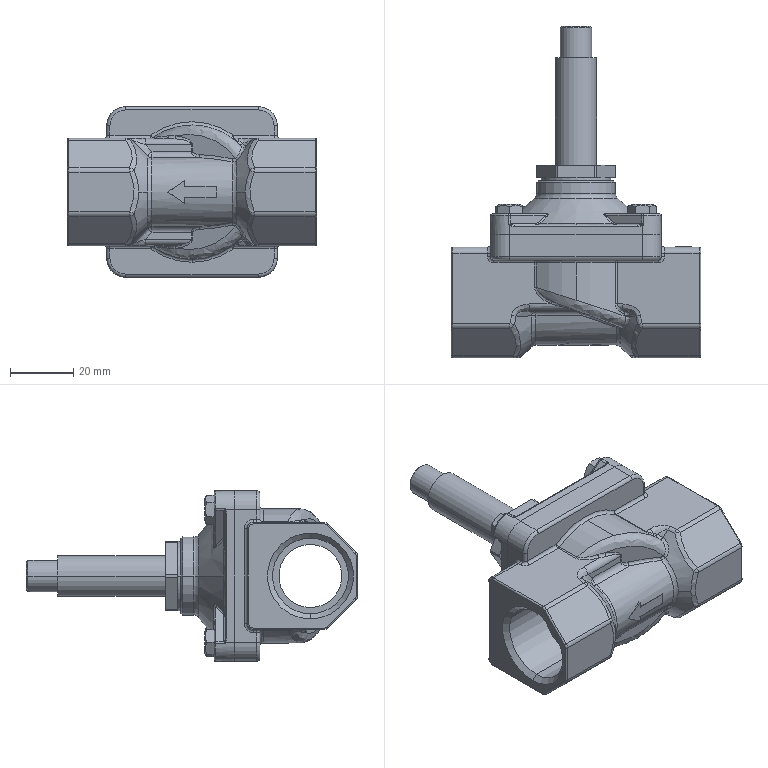Part | SolidWorks | features Boss 7, Fillet 6, Cut 5, Chamfer 3, CirPattern 2, Revolution 2, Extrusion 1, MirrorSolid 1, RefAxis 1, RevCut 1 | 7 solids | 458 faces | box 79 x 105 x 54 mm | volume 98145 mm3 | spline 135 | plane 117 | cylinder 114 | torus 56 | cone 22 | sphere 14 | commonest cylinder face diameters 1 x32 2 x31 4 x18 25 x9 12 x8 24 x4